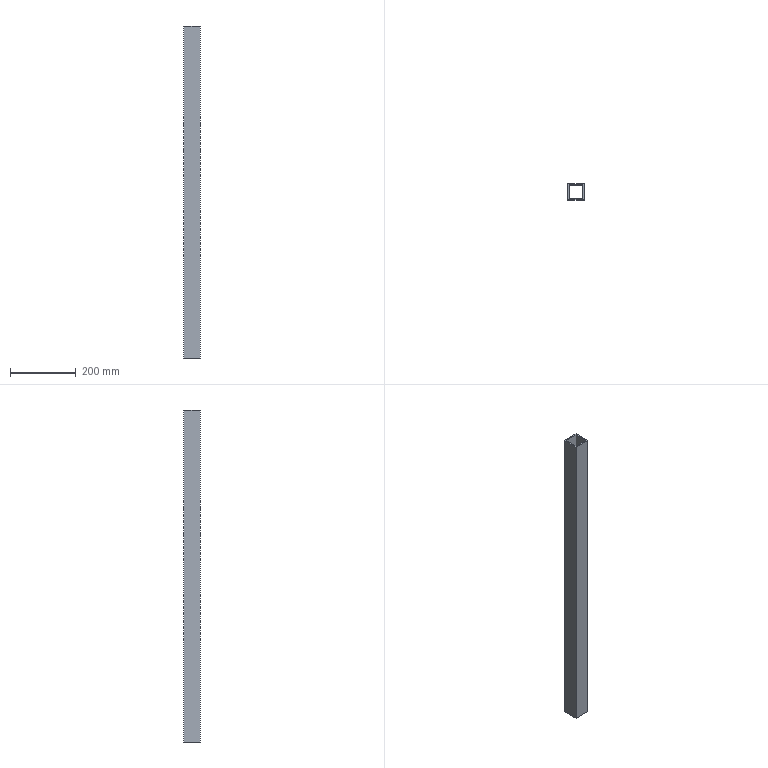Part | SolidWorks | features Extrusion 1 | 1 solid | 10 faces | box 50 x 50 x 1012 mm | volume 744832 mm3 | plane 10
STEP:
#1=CARTESIAN_POINT('',(-25.,25.,506.));
#2=VERTEX_POINT('',#1);
#3=CARTESIAN_POINT('',(-25.,-25.,506.));
#4=VERTEX_POINT('',#3);
#5=CARTESIAN_POINT('',(-25.,25.,506.));
#6=DIRECTION('',(0.,-1.,0.));
#7=VECTOR('',#6,1000.);
#8=LINE('',#5,#7);
#9=EDGE_CURVE('',#2,#4,#8,.T.);
#10=ORIENTED_EDGE('',*,*,#9,.F.);
#11=CARTESIAN_POINT('',(-25.,25.,-506.));
#12=VERTEX_POINT('',#11);
#13=CARTESIAN_POINT('',(-25.,25.,-506.));
#14=DIRECTION('',(0.,0.,1.));
#15=VECTOR('',#14,1000.);
#16=LINE('',#13,#15);
#17=EDGE_CURVE('',#12,#2,#16,.T.);
#18=ORIENTED_EDGE('',*,*,#17,.F.);
#19=CARTESIAN_POINT('',(-25.,-25.,-506.));
#20=VERTEX_POINT('',#19);
#21=CARTESIAN_POINT('',(-25.,25.,-506.));
#22=DIRECTION('',(0.,-1.,0.));
#23=VECTOR('',#22,1000.);
#24=LINE('',#21,#23);
#25=EDGE_CURVE('',#12,#20,#24,.T.);
#26=ORIENTED_EDGE('',*,*,#25,.T.);
#27=CARTESIAN_POINT('',(-25.,-25.,-506.));
#28=DIRECTION('',(0.,0.,1.));
#29=VECTOR('',#28,1000.);
#30=LINE('',#27,#29);
#31=EDGE_CURVE('',#20,#4,#30,.T.);
#32=ORIENTED_EDGE('',*,*,#31,.T.);
#33=EDGE_LOOP('',(#10,#18,#26,#32));
#34=FACE_OUTER_BOUND('',#33,.T.);
#35=CARTESIAN_POINT('',(-25.,25.,-506.));
#36=DIRECTION('',(-1.,0.,0.));
#37=DIRECTION('',(0.,0.,1.));
#38=AXIS2_PLACEMENT_3D('',#35,#36,#37);
#39=PLANE('',#38);
#40=ADVANCED_FACE('',(#34),#39,.T.);
#41=CARTESIAN_POINT('',(25.,25.,506.));
#42=VERTEX_POINT('',#41);
#43=CARTESIAN_POINT('',(25.,25.,506.));
#44=DIRECTION('',(-1.,0.,0.));
#45=VECTOR('',#44,1000.);
#46=LINE('',#43,#45);
#47=EDGE_CURVE('',#42,#2,#46,.T.);
#48=ORIENTED_EDGE('',*,*,#47,.F.);
#49=CARTESIAN_POINT('',(25.,25.,-506.));
#50=VERTEX_POINT('',#49);
#51=CARTESIAN_POINT('',(25.,25.,-506.));
#52=DIRECTION('',(0.,0.,1.));
#53=VECTOR('',#52,1000.);
#54=LINE('',#51,#53);
#55=EDGE_CURVE('',#50,#42,#54,.T.);
#56=ORIENTED_EDGE('',*,*,#55,.F.);
#57=CARTESIAN_POINT('',(25.,25.,-506.));
#58=DIRECTION('',(-1.,0.,0.));
#59=VECTOR('',#58,1000.);
#60=LINE('',#57,#59);
#61=EDGE_CURVE('',#50,#12,#60,.T.);
#62=ORIENTED_EDGE('',*,*,#61,.T.);
#63=ORIENTED_EDGE('',*,*,#17,.T.);
#64=EDGE_LOOP('',(#48,#56,#62,#63));
#65=FACE_OUTER_BOUND('',#64,.T.);
#66=CARTESIAN_POINT('',(25.,25.,-506.));
#67=DIRECTION('',(0.,1.,0.));
#68=DIRECTION('',(0.,0.,1.));
#69=AXIS2_PLACEMENT_3D('',#66,#67,#68);
#70=PLANE('',#69);
#71=ADVANCED_FACE('',(#65),#70,.T.);
#72=CARTESIAN_POINT('',(25.,-25.,506.));
#73=VERTEX_POINT('',#72);
#74=CARTESIAN_POINT('',(25.,-25.,506.));
#75=DIRECTION('',(0.,1.,0.));
#76=VECTOR('',#75,1000.);
#77=LINE('',#74,#76);
#78=EDGE_CURVE('',#73,#42,#77,.T.);
#79=ORIENTED_EDGE('',*,*,#78,.F.);
#80=CARTESIAN_POINT('',(25.,-25.,-506.));
#81=VERTEX_POINT('',#80);
#82=CARTESIAN_POINT('',(25.,-25.,-506.));
#83=DIRECTION('',(0.,0.,1.));
#84=VECTOR('',#83,1000.);
#85=LINE('',#82,#84);
#86=EDGE_CURVE('',#81,#73,#85,.T.);
#87=ORIENTED_EDGE('',*,*,#86,.F.);
#88=CARTESIAN_POINT('',(25.,-25.,-506.));
#89=DIRECTION('',(0.,1.,0.));
#90=VECTOR('',#89,1000.);
#91=LINE('',#88,#90);
#92=EDGE_CURVE('',#81,#50,#91,.T.);
#93=ORIENTED_EDGE('',*,*,#92,.T.);
#94=ORIENTED_EDGE('',*,*,#55,.T.);
#95=EDGE_LOOP('',(#79,#87,#93,#94));
#96=FACE_OUTER_BOUND('',#95,.T.);
#97=CARTESIAN_POINT('',(25.,-25.,-506.));
#98=DIRECTION('',(1.,0.,0.));
#99=DIRECTION('',(0.,0.,-1.));
#100=AXIS2_PLACEMENT_3D('',#97,#98,#99);
#101=PLANE('',#100);
#102=ADVANCED_FACE('',(#96),#101,.T.);
#103=CARTESIAN_POINT('',(-25.,-25.,506.));
#104=DIRECTION('',(1.,0.,0.));
#105=VECTOR('',#104,1000.);
#106=LINE('',#103,#105);
#107=EDGE_CURVE('',#4,#73,#106,.T.);
#108=ORIENTED_EDGE('',*,*,#107,.F.);
#109=ORIENTED_EDGE('',*,*,#31,.F.);
#110=CARTESIAN_POINT('',(-25.,-25.,-506.));
#111=DIRECTION('',(1.,0.,0.));
#112=VECTOR('',#111,1000.);
#113=LINE('',#110,#112);
#114=EDGE_CURVE('',#20,#81,#113,.T.);
#115=ORIENTED_EDGE('',*,*,#114,.T.);
#116=ORIENTED_EDGE('',*,*,#86,.T.);
#117=EDGE_LOOP('',(#108,#109,#115,#116));
#118=FACE_OUTER_BOUND('',#117,.T.);
#119=CARTESIAN_POINT('',(-25.,-25.,-506.));
#120=DIRECTION('',(0.,-1.,0.));
#121=DIRECTION('',(0.,0.,-1.));
#122=AXIS2_PLACEMENT_3D('',#119,#120,#121);
#123=PLANE('',#122);
#124=ADVANCED_FACE('',(#118),#123,.T.);
#125=CARTESIAN_POINT('',(21.,21.,-506.));
#126=VERTEX_POINT('',#125);
#127=CARTESIAN_POINT('',(-21.,21.,-506.));
#128=VERTEX_POINT('',#127);
#129=CARTESIAN_POINT('',(21.,21.,-506.));
#130=DIRECTION('',(-1.,0.,0.));
#131=VECTOR('',#130,1000.);
#132=LINE('',#129,#131);
#133=EDGE_CURVE('',#126,#128,#132,.T.);
#134=ORIENTED_EDGE('',*,*,#133,.T.);
#135=CARTESIAN_POINT('',(-21.,-21.,-506.));
#136=VERTEX_POINT('',#135);
#137=CARTESIAN_POINT('',(-21.,21.,-506.));
#138=DIRECTION('',(0.,-1.,0.));
#139=VECTOR('',#138,1000.);
#140=LINE('',#137,#139);
#141=EDGE_CURVE('',#128,#136,#140,.T.);
#142=ORIENTED_EDGE('',*,*,#141,.T.);
#143=CARTESIAN_POINT('',(21.,-21.,-506.));
#144=VERTEX_POINT('',#143);
#145=CARTESIAN_POINT('',(-21.,-21.,-506.));
#146=DIRECTION('',(1.,0.,0.));
#147=VECTOR('',#146,1000.);
#148=LINE('',#145,#147);
#149=EDGE_CURVE('',#136,#144,#148,.T.);
#150=ORIENTED_EDGE('',*,*,#149,.T.);
#151=CARTESIAN_POINT('',(21.,-21.,-506.));
#152=DIRECTION('',(0.,1.,0.));
#153=VECTOR('',#152,1000.);
#154=LINE('',#151,#153);
#155=EDGE_CURVE('',#144,#126,#154,.T.);
#156=ORIENTED_EDGE('',*,*,#155,.T.);
#157=EDGE_LOOP('',(#134,#142,#150,#156));
#158=FACE_BOUND('',#157,.T.);
#159=ORIENTED_EDGE('',*,*,#25,.F.);
#160=ORIENTED_EDGE('',*,*,#61,.F.);
#161=ORIENTED_EDGE('',*,*,#92,.F.);
#162=ORIENTED_EDGE('',*,*,#114,.F.);
#163=EDGE_LOOP('',(#159,#160,#161,#162));
#164=FACE_OUTER_BOUND('',#163,.T.);
#165=CARTESIAN_POINT('',(0.,0.,-506.));
#166=DIRECTION('',(0.,0.,1.));
#167=DIRECTION('',(1.,0.,0.));
#168=AXIS2_PLACEMENT_3D('',#165,#166,#167);
#169=PLANE('',#168);
#170=ADVANCED_FACE('',(#158,#164),#169,.F.);
#171=CARTESIAN_POINT('',(-21.,21.,506.));
#172=VERTEX_POINT('',#171);
#173=CARTESIAN_POINT('',(-21.,-21.,506.));
#174=VERTEX_POINT('',#173);
#175=CARTESIAN_POINT('',(-21.,21.,506.));
#176=DIRECTION('',(0.,-1.,0.));
#177=VECTOR('',#176,1000.);
#178=LINE('',#175,#177);
#179=EDGE_CURVE('',#172,#174,#178,.T.);
#180=ORIENTED_EDGE('',*,*,#179,.F.);
#181=CARTESIAN_POINT('',(21.,21.,506.));
#182=VERTEX_POINT('',#181);
#183=CARTESIAN_POINT('',(21.,21.,506.));
#184=DIRECTION('',(-1.,0.,0.));
#185=VECTOR('',#184,1000.);
#186=LINE('',#183,#185);
#187=EDGE_CURVE('',#182,#172,#186,.T.);
#188=ORIENTED_EDGE('',*,*,#187,.F.);
#189=CARTESIAN_POINT('',(21.,-21.,506.));
#190=VERTEX_POINT('',#189);
#191=CARTESIAN_POINT('',(21.,-21.,506.));
#192=DIRECTION('',(0.,1.,0.));
#193=VECTOR('',#192,1000.);
#194=LINE('',#191,#193);
#195=EDGE_CURVE('',#190,#182,#194,.T.);
#196=ORIENTED_EDGE('',*,*,#195,.F.);
#197=CARTESIAN_POINT('',(-21.,-21.,506.));
#198=DIRECTION('',(1.,0.,0.));
#199=VECTOR('',#198,1000.);
#200=LINE('',#197,#199);
#201=EDGE_CURVE('',#174,#190,#200,.T.);
#202=ORIENTED_EDGE('',*,*,#201,.F.);
#203=EDGE_LOOP('',(#180,#188,#196,#202));
#204=FACE_BOUND('',#203,.T.);
#205=ORIENTED_EDGE('',*,*,#9,.T.);
#206=ORIENTED_EDGE('',*,*,#107,.T.);
#207=ORIENTED_EDGE('',*,*,#78,.T.);
#208=ORIENTED_EDGE('',*,*,#47,.T.);
#209=EDGE_LOOP('',(#205,#206,#207,#208));
#210=FACE_OUTER_BOUND('',#209,.T.);
#211=CARTESIAN_POINT('',(0.,0.,506.));
#212=DIRECTION('',(0.,0.,1.));
#213=DIRECTION('',(1.,0.,0.));
#214=AXIS2_PLACEMENT_3D('',#211,#212,#213);
#215=PLANE('',#214);
#216=ADVANCED_FACE('',(#204,#210),#215,.T.);
#217=ORIENTED_EDGE('',*,*,#179,.T.);
#218=CARTESIAN_POINT('',(-21.,-21.,-506.));
#219=DIRECTION('',(0.,0.,1.));
#220=VECTOR('',#219,1000.);
#221=LINE('',#218,#220);
#222=EDGE_CURVE('',#136,#174,#221,.T.);
#223=ORIENTED_EDGE('',*,*,#222,.F.);
#224=ORIENTED_EDGE('',*,*,#141,.F.);
#225=CARTESIAN_POINT('',(-21.,21.,-506.));
#226=DIRECTION('',(0.,0.,1.));
#227=VECTOR('',#226,1000.);
#228=LINE('',#225,#227);
#229=EDGE_CURVE('',#128,#172,#228,.T.);
#230=ORIENTED_EDGE('',*,*,#229,.T.);
#231=EDGE_LOOP('',(#217,#223,#224,#230));
#232=FACE_OUTER_BOUND('',#231,.T.);
#233=CARTESIAN_POINT('',(-21.,21.,-506.));
#234=DIRECTION('',(-1.,0.,0.));
#235=DIRECTION('',(0.,0.,1.));
#236=AXIS2_PLACEMENT_3D('',#233,#234,#235);
#237=PLANE('',#236);
#238=ADVANCED_FACE('',(#232),#237,.F.);
#239=ORIENTED_EDGE('',*,*,#187,.T.);
#240=ORIENTED_EDGE('',*,*,#229,.F.);
#241=ORIENTED_EDGE('',*,*,#133,.F.);
#242=CARTESIAN_POINT('',(21.,21.,-506.));
#243=DIRECTION('',(0.,0.,1.));
#244=VECTOR('',#243,1000.);
#245=LINE('',#242,#244);
#246=EDGE_CURVE('',#126,#182,#245,.T.);
#247=ORIENTED_EDGE('',*,*,#246,.T.);
#248=EDGE_LOOP('',(#239,#240,#241,#247));
#249=FACE_OUTER_BOUND('',#248,.T.);
#250=CARTESIAN_POINT('',(21.,21.,-506.));
#251=DIRECTION('',(0.,1.,0.));
#252=DIRECTION('',(0.,0.,1.));
#253=AXIS2_PLACEMENT_3D('',#250,#251,#252);
#254=PLANE('',#253);
#255=ADVANCED_FACE('',(#249),#254,.F.);
#256=ORIENTED_EDGE('',*,*,#195,.T.);
#257=ORIENTED_EDGE('',*,*,#246,.F.);
#258=ORIENTED_EDGE('',*,*,#155,.F.);
#259=CARTESIAN_POINT('',(21.,-21.,-506.));
#260=DIRECTION('',(0.,0.,1.));
#261=VECTOR('',#260,1000.);
#262=LINE('',#259,#261);
#263=EDGE_CURVE('',#144,#190,#262,.T.);
#264=ORIENTED_EDGE('',*,*,#263,.T.);
#265=EDGE_LOOP('',(#256,#257,#258,#264));
#266=FACE_OUTER_BOUND('',#265,.T.);
#267=CARTESIAN_POINT('',(21.,-21.,-506.));
#268=DIRECTION('',(1.,0.,0.));
#269=DIRECTION('',(0.,0.,-1.));
#270=AXIS2_PLACEMENT_3D('',#267,#268,#269);
#271=PLANE('',#270);
#272=ADVANCED_FACE('',(#266),#271,.F.);
#273=ORIENTED_EDGE('',*,*,#201,.T.);
#274=ORIENTED_EDGE('',*,*,#263,.F.);
#275=ORIENTED_EDGE('',*,*,#149,.F.);
#276=ORIENTED_EDGE('',*,*,#222,.T.);
#277=EDGE_LOOP('',(#273,#274,#275,#276));
#278=FACE_OUTER_BOUND('',#277,.T.);
#279=CARTESIAN_POINT('',(-21.,-21.,-506.));
#280=DIRECTION('',(0.,-1.,0.));
#281=DIRECTION('',(0.,0.,-1.));
#282=AXIS2_PLACEMENT_3D('',#279,#280,#281);
#283=PLANE('',#282);
#284=ADVANCED_FACE('',(#278),#283,.F.);
#285=CLOSED_SHELL('',(#40,#71,#102,#124,#170,#216,#238,#255,#272,#284));
#286=MANIFOLD_SOLID_BREP('',#285);
#287=CARTESIAN_POINT('',(0.,0.,0.));
#288=DIRECTION('',(0.,0.,1.));
#289=DIRECTION('',(1.,0.,0.));
#290=AXIS2_PLACEMENT_3D('',#287,#288,#289);
#291=(LENGTH_UNIT()NAMED_UNIT(*)SI_UNIT(.MILLI.,.METRE.));
#292=UNCERTAINTY_MEASURE_WITH_UNIT(LENGTH_MEASURE(0.00001),#291,'','');
#293=(NAMED_UNIT(*)PLANE_ANGLE_UNIT()SI_UNIT($,.RADIAN.));
#294=(NAMED_UNIT(*)SI_UNIT($,.STERADIAN.)SOLID_ANGLE_UNIT());
#295=(GEOMETRIC_REPRESENTATION_CONTEXT(3)GLOBAL_UNCERTAINTY_ASSIGNED_CONTEXT((#292))GLOBAL_UNIT_ASSIGNED_CONTEXT((#291,#293,#294))REPRESENTATION_CONTEXT('',''));
#296=ADVANCED_BREP_SHAPE_REPRESENTATION('',(#286,#290),#295);